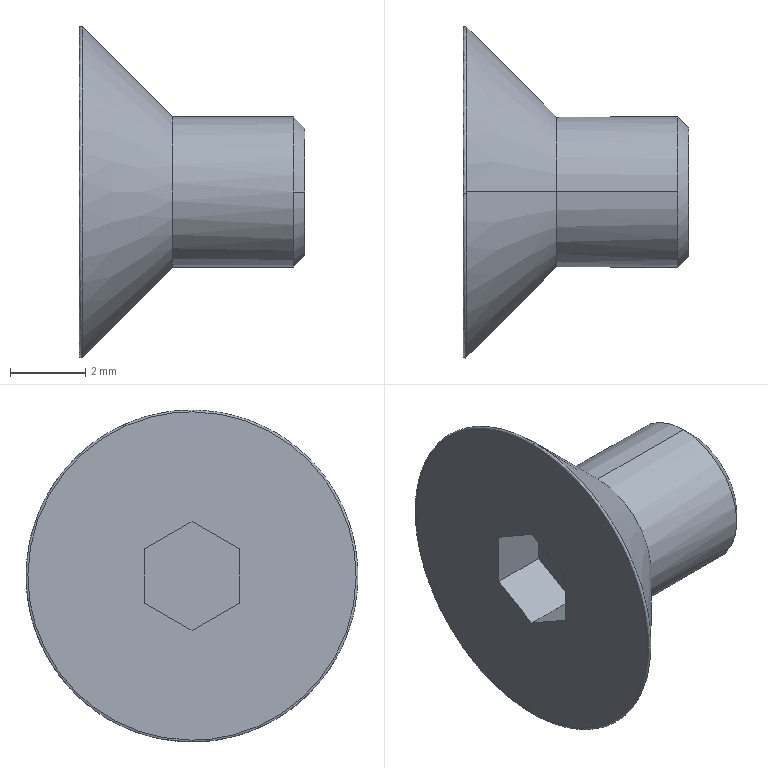Part | STEP file | M4-6-1 | 1 solid | 17 faces | box 6 x 8.819 x 8.819 mm | volume 121.278 mm3 | plane 9 | cone 4 | spline 2 | cylinder 2 | commonest cylinder face diameters 4 x2